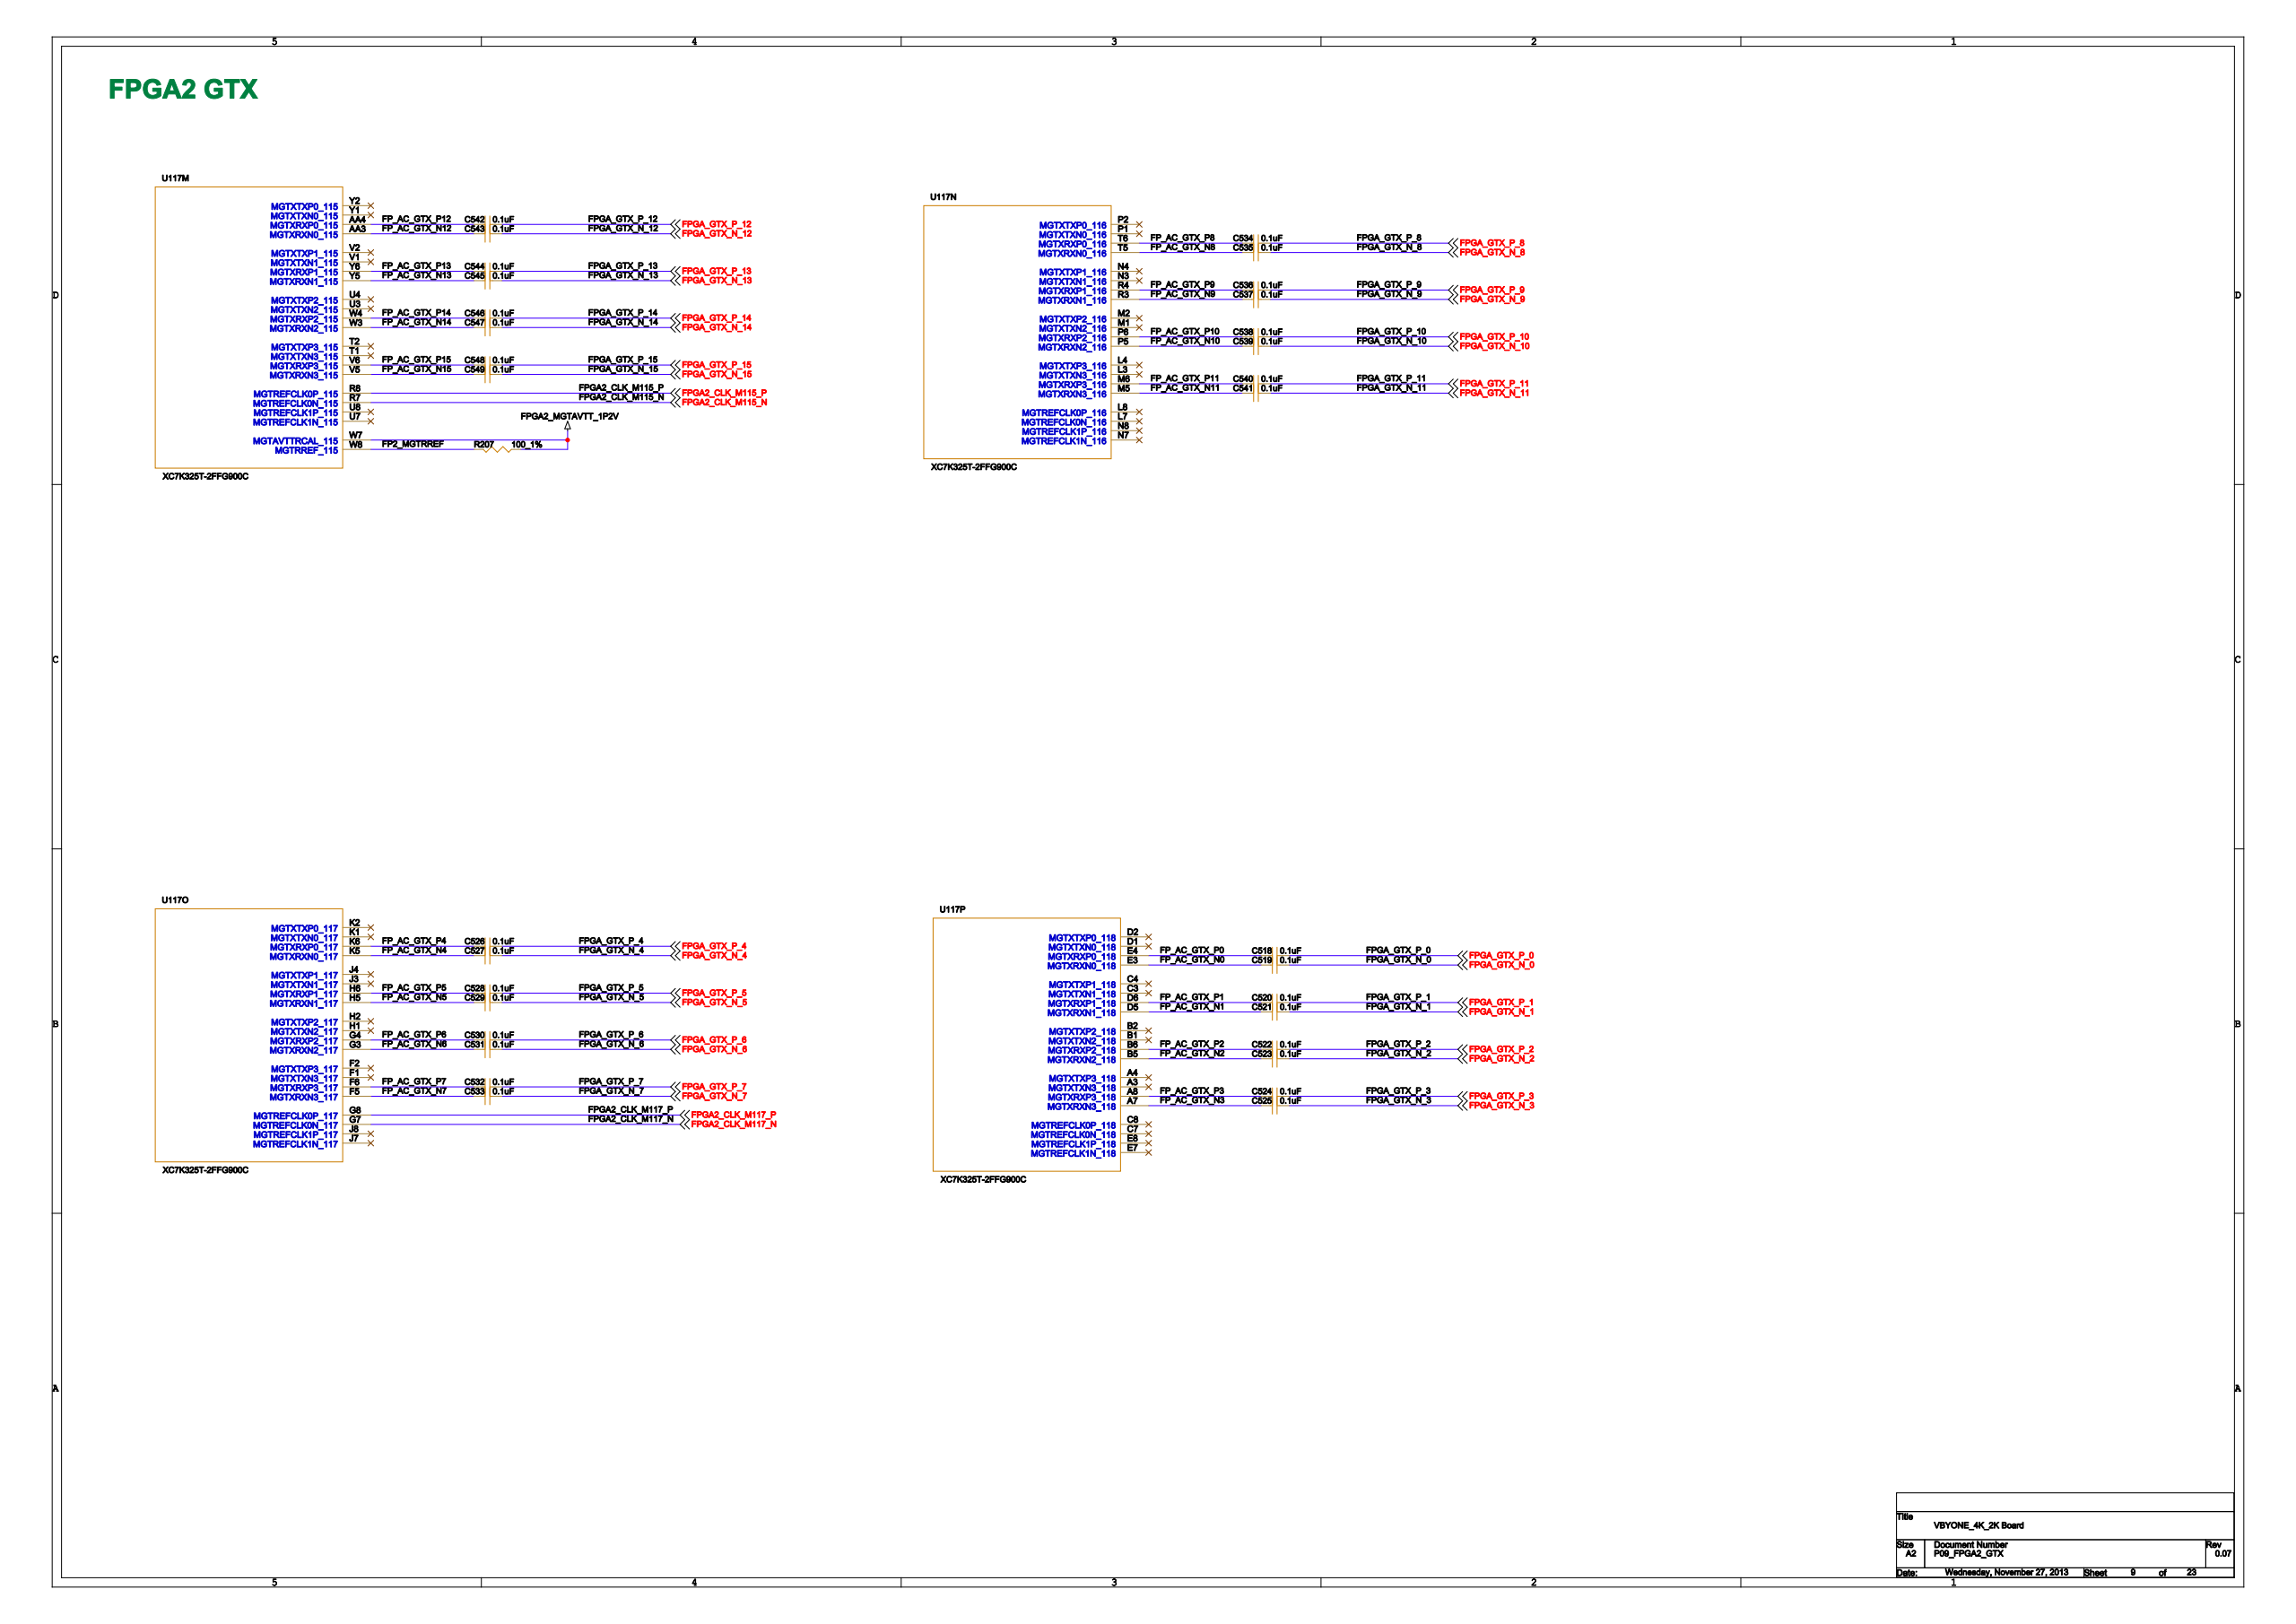Circuit board | Cadence Allegro | 1712 parts | 1495 nets | one sheet of the schematic
Parts on this sheet (reference | value | footprint):
C518 | 0.1uF | CRC1005RZAS
C519 | 0.1uF | CRC1005RZAS
C520 | 0.1uF | CRC1005RZAS
C521 | 0.1uF | CRC1005RZAS
C522 | 0.1uF | CRC1005RZAS
C523 | 0.1uF | CRC1005RZAS
C524 | 0.1uF | CRC1005RZAS
C525 | 0.1uF | CRC1005RZAS
C526 | 0.1uF | CRC1005RZAS
C527 | 0.1uF | CRC1005RZAS
C528 | 0.1uF | CRC1005RZAS
C529 | 0.1uF | CRC1005RZAS
C530 | 0.1uF | CRC1005RZAS
C531 | 0.1uF | CRC1005RZAS
C532 | 0.1uF | CRC1005RZAS
C533 | 0.1uF | CRC1005RZAS
C534 | 0.1uF | CRC1005RZAS
C535 | 0.1uF | CRC1005RZAS
C536 | 0.1uF | CRC1005RZAS
C537 | 0.1uF | CRC1005RZAS
C538 | 0.1uF | CRC1005RZAS
C539 | 0.1uF | CRC1005RZAS
C540 | 0.1uF | CRC1005RZAS
C541 | 0.1uF | CRC1005RZAS
C542 | 0.1uF | CRC1005RZAS
C543 | 0.1uF | CRC1005RZAS
C544 | 0.1uF | CRC1005RZAS
C545 | 0.1uF | CRC1005RZAS
C546 | 0.1uF | CRC1005RZAS
C547 | 0.1uF | CRC1005RZAS
C548 | 0.1uF | CRC1005RZAS
C549 | 0.1uF | CRC1005RZAS
R207 | 100_1% | CRC1005RZAS
U117 | XC7K325T-2FFG900C | BGA900RGAS
Nets of these parts (net: part-pin ...):
FPGA2_MGTAVTT_1P2V: R207-1 U117-W7
FPGA2_CLK_M115_P: U117-R8
FPGA2_CLK_M115_N: U117-R7
FPGA2_CLK_M117_P: U117-G8
FPGA2_CLK_M117_N: U117-G7
FP_AC_GTX_P0: C518-1 U117-E4
FPGA_GTX_P_0: C518-2
FP_AC_GTX_N0: C519-1 U117-E3
FPGA_GTX_N_0: C519-2
FP_AC_GTX_P1: C520-1 U117-D6
FPGA_GTX_P_1: C520-2
FP_AC_GTX_N1: C521-1 U117-D5
FPGA_GTX_N_1: C521-2
FP_AC_GTX_P2: C522-1 U117-B6
FPGA_GTX_P_2: C522-2
FP_AC_GTX_N2: C523-1 U117-B5
FPGA_GTX_N_2: C523-2
FP_AC_GTX_P3: C524-1 U117-A8
FPGA_GTX_P_3: C524-2
FP_AC_GTX_N3: C525-1 U117-A7
FPGA_GTX_N_3: C525-2
FP_AC_GTX_P4: C526-1 U117-K6
FPGA_GTX_P_4: C526-2
FP_AC_GTX_N4: C527-1 U117-K5
FPGA_GTX_N_4: C527-2
FP_AC_GTX_P5: C528-1 U117-H6
FPGA_GTX_P_5: C528-2
FP_AC_GTX_N5: C529-1 U117-H5
FPGA_GTX_N_5: C529-2
FP_AC_GTX_P6: C530-1 U117-G4
FPGA_GTX_P_6: C530-2
FP_AC_GTX_N6: C531-1 U117-G3
FPGA_GTX_N_6: C531-2
FP_AC_GTX_P7: C532-1 U117-F6
FPGA_GTX_P_7: C532-2
FP_AC_GTX_N7: C533-1 U117-F5
FPGA_GTX_N_7: C533-2
FP_AC_GTX_P8: C534-1 U117-T6
FPGA_GTX_P_8: C534-2
FP_AC_GTX_N8: C535-1 U117-T5
FPGA_GTX_N_8: C535-2
FP_AC_GTX_P9: C536-1 U117-R4
FPGA_GTX_P_9: C536-2
FP_AC_GTX_N9: C537-1 U117-R3
FPGA_GTX_N_9: C537-2
FP_AC_GTX_P10: C538-1 U117-P6
FPGA_GTX_P_10: C538-2
FP_AC_GTX_N10: C539-1 U117-P5
FPGA_GTX_N_10: C539-2
FP_AC_GTX_P11: C540-1 U117-M6
FPGA_GTX_P_11: C540-2
FP_AC_GTX_N11: C541-1 U117-M5
FPGA_GTX_N_11: C541-2
FP_AC_GTX_P12: C542-1 U117-AA4
FPGA_GTX_P_12: C542-2
FP_AC_GTX_N12: C543-1 U117-AA3
FPGA_GTX_N_12: C543-2
FP_AC_GTX_P13: C544-1 U117-Y6
FPGA_GTX_P_13: C544-2
FP_AC_GTX_N13: C545-1 U117-Y5
FPGA_GTX_N_13: C545-2
FP_AC_GTX_P14: C546-1 U117-W4
FPGA_GTX_P_14: C546-2
FP_AC_GTX_N14: C547-1 U117-W3
FPGA_GTX_N_14: C547-2
FP_AC_GTX_P15: C548-1 U117-V6
FPGA_GTX_P_15: C548-2
FP_AC_GTX_N15: C549-1 U117-V5
FPGA_GTX_N_15: C549-2
FP2_MGTRREF: R207-2 U117-W8